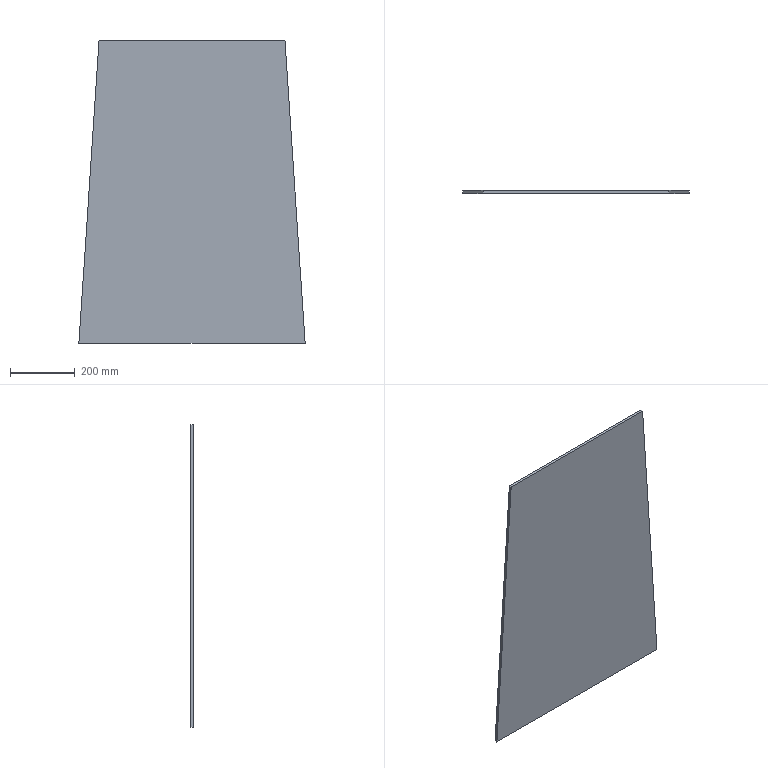Part | SolidWorks | features FlatPattern 1, SMBaseFlange 1, SheetMetal 1 | 1 solid | 6 faces | box 700 x 8 x 935 mm | volume 4768500 mm3 | plane 6
STEP:
#1=CARTESIAN_POINT('',(0.,0.,0.));
#2=VERTEX_POINT('',#1);
#3=CARTESIAN_POINT('',(62.5,0.,935.));
#4=VERTEX_POINT('',#3);
#5=CARTESIAN_POINT('',(62.5,0.,935.));
#6=DIRECTION('',(0.0667,0.,0.9978));
#7=VECTOR('',#6,1000.);
#8=LINE('',#5,#7);
#9=EDGE_CURVE('',#2,#4,#8,.T.);
#10=ORIENTED_EDGE('',*,*,#9,.F.);
#11=CARTESIAN_POINT('',(0.,-8.,0.));
#12=VERTEX_POINT('',#11);
#13=CARTESIAN_POINT('',(0.,-8.,0.));
#14=DIRECTION('',(0.,1.,0.));
#15=VECTOR('',#14,1000.);
#16=LINE('',#13,#15);
#17=EDGE_CURVE('',#12,#2,#16,.T.);
#18=ORIENTED_EDGE('',*,*,#17,.F.);
#19=CARTESIAN_POINT('',(62.5,-8.,935.));
#20=VERTEX_POINT('',#19);
#21=CARTESIAN_POINT('',(62.5,-8.,935.));
#22=DIRECTION('',(0.0667,0.,0.9978));
#23=VECTOR('',#22,1000.);
#24=LINE('',#21,#23);
#25=EDGE_CURVE('',#12,#20,#24,.T.);
#26=ORIENTED_EDGE('',*,*,#25,.T.);
#27=CARTESIAN_POINT('',(62.5,-8.,935.));
#28=DIRECTION('',(0.,1.,0.));
#29=VECTOR('',#28,1000.);
#30=LINE('',#27,#29);
#31=EDGE_CURVE('',#20,#4,#30,.T.);
#32=ORIENTED_EDGE('',*,*,#31,.T.);
#33=EDGE_LOOP('',(#10,#18,#26,#32));
#34=FACE_OUTER_BOUND('',#33,.T.);
#35=CARTESIAN_POINT('',(62.5,-8.,935.));
#36=DIRECTION('',(-0.9978,0.,0.0667));
#37=DIRECTION('',(0.0667,0.,0.9978));
#38=AXIS2_PLACEMENT_3D('',#35,#36,#37);
#39=PLANE('',#38);
#40=ADVANCED_FACE('',(#34),#39,.T.);
#41=CARTESIAN_POINT('',(700.,0.,0.));
#42=VERTEX_POINT('',#41);
#43=CARTESIAN_POINT('',(0.,0.,0.));
#44=DIRECTION('',(-1.,0.,0.));
#45=VECTOR('',#44,1000.);
#46=LINE('',#43,#45);
#47=EDGE_CURVE('',#42,#2,#46,.T.);
#48=ORIENTED_EDGE('',*,*,#47,.F.);
#49=CARTESIAN_POINT('',(700.,-8.,0.));
#50=VERTEX_POINT('',#49);
#51=CARTESIAN_POINT('',(700.,-8.,0.));
#52=DIRECTION('',(0.,1.,0.));
#53=VECTOR('',#52,1000.);
#54=LINE('',#51,#53);
#55=EDGE_CURVE('',#50,#42,#54,.T.);
#56=ORIENTED_EDGE('',*,*,#55,.F.);
#57=CARTESIAN_POINT('',(0.,-8.,0.));
#58=DIRECTION('',(-1.,0.,0.));
#59=VECTOR('',#58,1000.);
#60=LINE('',#57,#59);
#61=EDGE_CURVE('',#50,#12,#60,.T.);
#62=ORIENTED_EDGE('',*,*,#61,.T.);
#63=ORIENTED_EDGE('',*,*,#17,.T.);
#64=EDGE_LOOP('',(#48,#56,#62,#63));
#65=FACE_OUTER_BOUND('',#64,.T.);
#66=CARTESIAN_POINT('',(0.,-8.,0.));
#67=DIRECTION('',(0.,0.,-1.));
#68=DIRECTION('',(-1.,0.,0.));
#69=AXIS2_PLACEMENT_3D('',#66,#67,#68);
#70=PLANE('',#69);
#71=ADVANCED_FACE('',(#65),#70,.T.);
#72=CARTESIAN_POINT('',(637.5,0.,935.));
#73=VERTEX_POINT('',#72);
#74=CARTESIAN_POINT('',(700.,0.,0.));
#75=DIRECTION('',(0.0667,0.,-0.9978));
#76=VECTOR('',#75,1000.);
#77=LINE('',#74,#76);
#78=EDGE_CURVE('',#73,#42,#77,.T.);
#79=ORIENTED_EDGE('',*,*,#78,.F.);
#80=CARTESIAN_POINT('',(637.5,-8.,935.));
#81=VERTEX_POINT('',#80);
#82=CARTESIAN_POINT('',(637.5,-8.,935.));
#83=DIRECTION('',(0.,1.,0.));
#84=VECTOR('',#83,1000.);
#85=LINE('',#82,#84);
#86=EDGE_CURVE('',#81,#73,#85,.T.);
#87=ORIENTED_EDGE('',*,*,#86,.F.);
#88=CARTESIAN_POINT('',(700.,-8.,0.));
#89=DIRECTION('',(0.0667,0.,-0.9978));
#90=VECTOR('',#89,1000.);
#91=LINE('',#88,#90);
#92=EDGE_CURVE('',#81,#50,#91,.T.);
#93=ORIENTED_EDGE('',*,*,#92,.T.);
#94=ORIENTED_EDGE('',*,*,#55,.T.);
#95=EDGE_LOOP('',(#79,#87,#93,#94));
#96=FACE_OUTER_BOUND('',#95,.T.);
#97=CARTESIAN_POINT('',(700.,-8.,0.));
#98=DIRECTION('',(0.9978,0.,0.0667));
#99=DIRECTION('',(0.0667,0.,-0.9978));
#100=AXIS2_PLACEMENT_3D('',#97,#98,#99);
#101=PLANE('',#100);
#102=ADVANCED_FACE('',(#96),#101,.T.);
#103=CARTESIAN_POINT('',(637.5,0.,935.));
#104=DIRECTION('',(1.,0.,0.));
#105=VECTOR('',#104,1000.);
#106=LINE('',#103,#105);
#107=EDGE_CURVE('',#4,#73,#106,.T.);
#108=ORIENTED_EDGE('',*,*,#107,.F.);
#109=ORIENTED_EDGE('',*,*,#31,.F.);
#110=CARTESIAN_POINT('',(637.5,-8.,935.));
#111=DIRECTION('',(1.,0.,0.));
#112=VECTOR('',#111,1000.);
#113=LINE('',#110,#112);
#114=EDGE_CURVE('',#20,#81,#113,.T.);
#115=ORIENTED_EDGE('',*,*,#114,.T.);
#116=ORIENTED_EDGE('',*,*,#86,.T.);
#117=EDGE_LOOP('',(#108,#109,#115,#116));
#118=FACE_OUTER_BOUND('',#117,.T.);
#119=CARTESIAN_POINT('',(637.5,-8.,935.));
#120=DIRECTION('',(0.,0.,1.));
#121=DIRECTION('',(1.,0.,0.));
#122=AXIS2_PLACEMENT_3D('',#119,#120,#121);
#123=PLANE('',#122);
#124=ADVANCED_FACE('',(#118),#123,.T.);
#125=ORIENTED_EDGE('',*,*,#25,.F.);
#126=ORIENTED_EDGE('',*,*,#61,.F.);
#127=ORIENTED_EDGE('',*,*,#92,.F.);
#128=ORIENTED_EDGE('',*,*,#114,.F.);
#129=EDGE_LOOP('',(#125,#126,#127,#128));
#130=FACE_OUTER_BOUND('',#129,.T.);
#131=CARTESIAN_POINT('',(0.,-8.,0.));
#132=DIRECTION('',(0.,-1.,0.));
#133=DIRECTION('',(0.,0.,-1.));
#134=AXIS2_PLACEMENT_3D('',#131,#132,#133);
#135=PLANE('',#134);
#136=ADVANCED_FACE('',(#130),#135,.T.);
#137=ORIENTED_EDGE('',*,*,#9,.T.);
#138=ORIENTED_EDGE('',*,*,#107,.T.);
#139=ORIENTED_EDGE('',*,*,#78,.T.);
#140=ORIENTED_EDGE('',*,*,#47,.T.);
#141=EDGE_LOOP('',(#137,#138,#139,#140));
#142=FACE_OUTER_BOUND('',#141,.T.);
#143=CARTESIAN_POINT('',(0.,0.,0.));
#144=DIRECTION('',(0.,-1.,0.));
#145=DIRECTION('',(0.,0.,-1.));
#146=AXIS2_PLACEMENT_3D('',#143,#144,#145);
#147=PLANE('',#146);
#148=ADVANCED_FACE('',(#142),#147,.F.);
#149=CLOSED_SHELL('',(#40,#71,#102,#124,#136,#148));
#150=MANIFOLD_SOLID_BREP('',#149);
#151=CARTESIAN_POINT('',(0.,0.,0.));
#152=DIRECTION('',(0.,0.,1.));
#153=DIRECTION('',(1.,0.,0.));
#154=AXIS2_PLACEMENT_3D('',#151,#152,#153);
#155=(LENGTH_UNIT()NAMED_UNIT(*)SI_UNIT(.MILLI.,.METRE.));
#156=UNCERTAINTY_MEASURE_WITH_UNIT(LENGTH_MEASURE(0.00001),#155,'','');
#157=(NAMED_UNIT(*)PLANE_ANGLE_UNIT()SI_UNIT($,.RADIAN.));
#158=(NAMED_UNIT(*)SI_UNIT($,.STERADIAN.)SOLID_ANGLE_UNIT());
#159=(GEOMETRIC_REPRESENTATION_CONTEXT(3)GLOBAL_UNCERTAINTY_ASSIGNED_CONTEXT((#156))GLOBAL_UNIT_ASSIGNED_CONTEXT((#155,#157,#158))REPRESENTATION_CONTEXT('',''));
#160=ADVANCED_BREP_SHAPE_REPRESENTATION('',(#150,#154),#159);